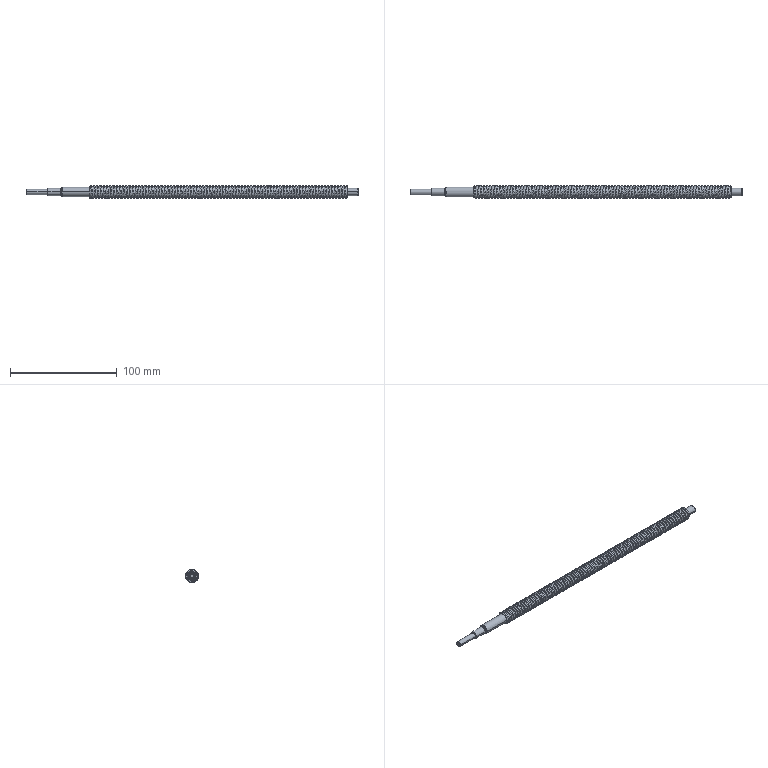Part | Creo | features DATUM PLANE 3, COORDINATE SYSTEM 1, CURVE 1, CUT 1, PROTRUSION 1 | 1 solid | 208 faces | box 310.5 x 12.006 x 12.001 mm | volume 25764 mm3 | cylinder 170 | spline 21 | cone 10 | plane 7 | commonest cylinder face diameters 12 x160 7 x4 5 x2 6 x2 9 x2